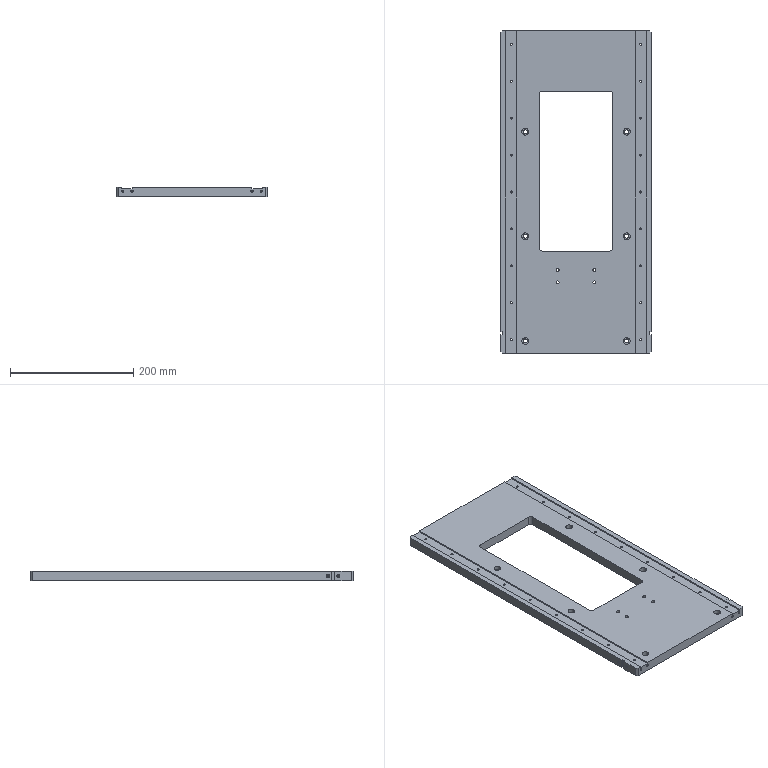Part | SolidWorks | features BaseBody 1 | 1 solid | 140 faces | box 245 x 524 x 15 mm | volume 1411431 mm3 | cylinder 88 | plane 36 | cone 16 | commonest cylinder face diameters 3.3 x44 5 x16 6.6 x12 11 x12 10 x4